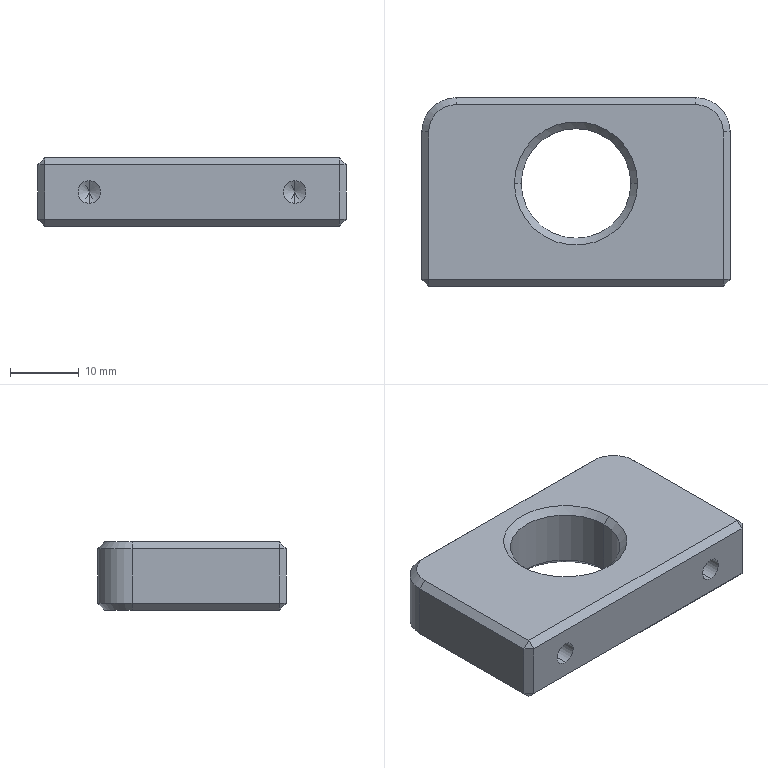Part | STEP file | 1 solid | 40 faces | box 45 x 27.5 x 10 mm | volume 9795 mm3 | plane 20 | cone 12 | cylinder 8 | commonest cylinder face diameters 3.3 x4 10 x2 16 x2